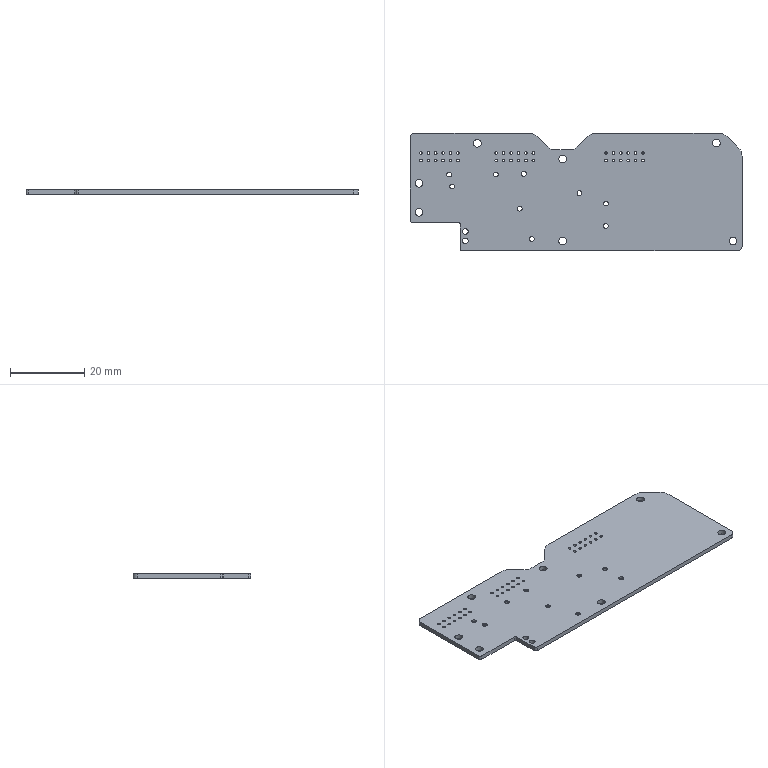Part | STEP file | 推动功放控制1PCB | 1 solid | 285 faces | box 89.69 x 31.78 x 1.2 mm | volume 3157 mm3 | plane 229 | cylinder 56 | commonest cylinder face diameters 0.7 x36 2.1 x7 6.132 x6 1.5 x2 2.54 x2 0.796 x1